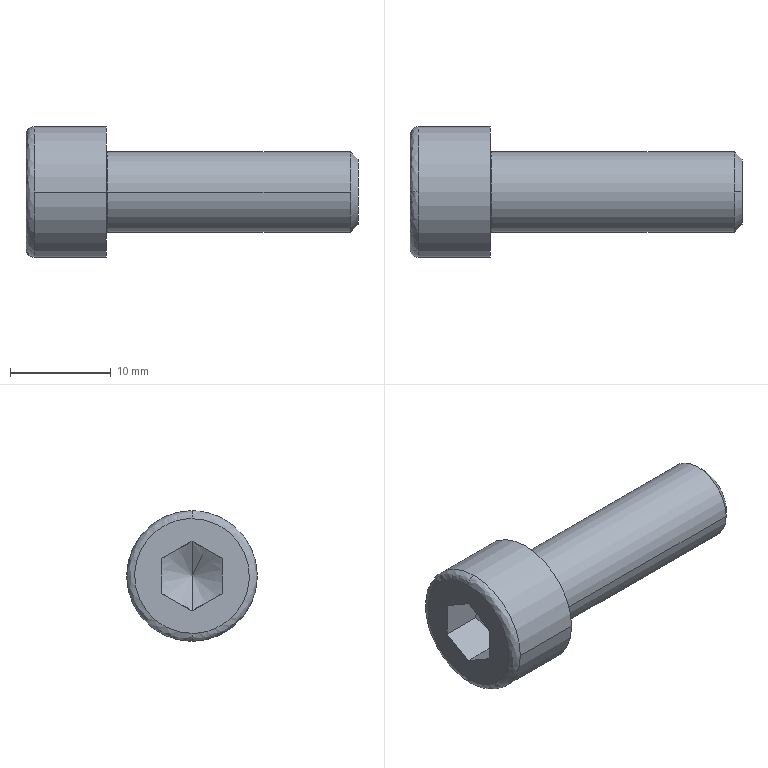Part | SolidWorks | features BaseBody 1 | 1 solid | 21 faces | box 33 x 13 x 13 mm | volume 2157 mm3 | plane 9 | spline 4 | cylinder 4 | cone 4 | commonest cylinder face diameters 8 x2 13 x2
STEP:
#1=CARTESIAN_POINT('',(0.,0.,4.1));
#2=VERTEX_POINT('',#1);
#3=CARTESIAN_POINT('',(0.,0.,-4.1));
#4=VERTEX_POINT('',#3);
#5=CARTESIAN_POINT('',(0.,0.,4.1));
#6=CARTESIAN_POINT('',(0.,0.2605,4.1));
#7=CARTESIAN_POINT('',(0.,0.6445,4.064));
#8=CARTESIAN_POINT('',(0.,1.081,3.959));
#9=CARTESIAN_POINT('',(0.,1.296,3.891));
#10=CARTESIAN_POINT('',(0.,1.388,3.858));
#11=CARTESIAN_POINT('',(0.,1.448,3.836));
#12=CARTESIAN_POINT('',(0.,1.477,3.825));
#13=CARTESIAN_POINT('',(0.,1.638,3.761));
#14=CARTESIAN_POINT('',(0.,1.826,3.675));
#15=CARTESIAN_POINT('',(0.,2.007,3.576));
#16=CARTESIAN_POINT('',(0.,2.127,3.506));
#17=CARTESIAN_POINT('',(0.,2.184,3.47));
#18=CARTESIAN_POINT('',(0.,2.48,3.277));
#19=CARTESIAN_POINT('',(0.,2.699,3.099));
#20=CARTESIAN_POINT('',(0.,2.999,2.799));
#21=CARTESIAN_POINT('',(0.,3.141,2.642));
#22=CARTESIAN_POINT('',(0.,3.27,2.475));
#23=CARTESIAN_POINT('',(0.,3.353,2.361));
#24=CARTESIAN_POINT('',(0.,3.394,2.301));
#25=CARTESIAN_POINT('',(0.,3.507,2.128));
#26=CARTESIAN_POINT('',(0.,3.612,1.949));
#27=CARTESIAN_POINT('',(0.,3.717,1.732));
#28=CARTESIAN_POINT('',(0.,3.759,1.637));
#29=CARTESIAN_POINT('',(0.,3.786,1.573));
#30=CARTESIAN_POINT('',(0.,3.8,1.539));
#31=CARTESIAN_POINT('',(0.,4.004,1.024));
#32=CARTESIAN_POINT('',(0.,4.1,0.5212));
#33=CARTESIAN_POINT('',(0.,4.1,-0.2606));
#34=CARTESIAN_POINT('',(0.,4.076,-0.5169));
#35=CARTESIAN_POINT('',(0.,4.004,-0.8942));
#36=CARTESIAN_POINT('',(0.,3.959,-1.081));
#37=CARTESIAN_POINT('',(0.,3.891,-1.296));
#38=CARTESIAN_POINT('',(0.,3.858,-1.388));
#39=CARTESIAN_POINT('',(0.,3.836,-1.449));
#40=CARTESIAN_POINT('',(0.,3.825,-1.477));
#41=CARTESIAN_POINT('',(0.,3.761,-1.638));
#42=CARTESIAN_POINT('',(0.,3.675,-1.826));
#43=CARTESIAN_POINT('',(0.,3.576,-2.007));
#44=CARTESIAN_POINT('',(0.,3.506,-2.127));
#45=CARTESIAN_POINT('',(0.,3.47,-2.184));
#46=CARTESIAN_POINT('',(0.,3.277,-2.48));
#47=CARTESIAN_POINT('',(0.,3.099,-2.699));
#48=CARTESIAN_POINT('',(0.,2.799,-2.999));
#49=CARTESIAN_POINT('',(0.,2.642,-3.141));
#50=CARTESIAN_POINT('',(0.,2.475,-3.27));
#51=CARTESIAN_POINT('',(0.,2.361,-3.353));
#52=CARTESIAN_POINT('',(0.,2.301,-3.394));
#53=CARTESIAN_POINT('',(0.,2.128,-3.507));
#54=CARTESIAN_POINT('',(0.,1.949,-3.612));
#55=CARTESIAN_POINT('',(0.,1.732,-3.717));
#56=CARTESIAN_POINT('',(0.,1.637,-3.759));
#57=CARTESIAN_POINT('',(0.,1.573,-3.786));
#58=CARTESIAN_POINT('',(0.,1.539,-3.8));
#59=CARTESIAN_POINT('',(0.,1.025,-4.004));
#60=CARTESIAN_POINT('',(0.,0.521,-4.1));
#61=CARTESIAN_POINT('',(0.,0.,-4.1));
#62=B_SPLINE_CURVE_WITH_KNOTS('',3,(#5,#6,#7,#8,#9,#10,#11,#12,#13,#14,#15,#16,#17,#18,#19,#20,#21,#22,#23,#24,#25,#26,#27,#28,#29,#30,#31,#32,#33,#34,#35,#36,#37,#38,#39,#40,#41,#42,#43,#44,#45,#46,#47,#48,#49,#50,#51,#52,#53,#54,#55,#56,#57,#58,#59,#60,#61),.UNSPECIFIED.,.F.,.F.,(4,1,1,1,2,2,1,2,2,2,1,2,2,1,1,2,2,2,2,1,1,2,2,1,2,2,2,1,2,2,1,1,2,2,4),(0.75,0.7813,0.7969,0.8047,0.8086,0.8125,0.8281,0.8359,0.8438,0.875,0.8906,0.8984,0.9063,0.9219,0.9297,0.9336,0.9375,1.,1.031,1.047,1.055,1.059,1.062,1.078,1.086,1.094,1.125,1.141,1.148,1.156,1.172,1.18,1.184,1.187,1.25),.UNSPECIFIED.);
#63=EDGE_CURVE('',#2,#4,#62,.T.);
#64=ORIENTED_EDGE('',*,*,#63,.F.);
#65=CARTESIAN_POINT('',(0.1,0.,4.));
#66=VERTEX_POINT('',#65);
#67=CARTESIAN_POINT('',(0.1,0.,4.1));
#68=DIRECTION('',(0.,-1.,0.));
#69=DIRECTION('',(0.,0.,1.));
#70=AXIS2_PLACEMENT_3D('',#67,#68,#69);
#71=CIRCLE('',#70,0.1);
#72=EDGE_CURVE('',#2,#66,#71,.T.);
#73=ORIENTED_EDGE('',*,*,#72,.T.);
#74=CARTESIAN_POINT('',(0.1,4.,0.));
#75=VERTEX_POINT('',#74);
#76=CARTESIAN_POINT('',(0.1,0.,0.));
#77=DIRECTION('',(1.,0.,0.));
#78=DIRECTION('',(0.,1.,0.));
#79=AXIS2_PLACEMENT_3D('',#76,#77,#78);
#80=CIRCLE('',#79,4.);
#81=EDGE_CURVE('',#75,#66,#80,.T.);
#82=ORIENTED_EDGE('',*,*,#81,.F.);
#83=CARTESIAN_POINT('',(0.1,0.,-4.));
#84=VERTEX_POINT('',#83);
#85=CARTESIAN_POINT('',(0.1,0.,0.));
#86=DIRECTION('',(1.,0.,0.));
#87=DIRECTION('',(0.,1.,0.));
#88=AXIS2_PLACEMENT_3D('',#85,#86,#87);
#89=CIRCLE('',#88,4.);
#90=EDGE_CURVE('',#84,#75,#89,.T.);
#91=ORIENTED_EDGE('',*,*,#90,.F.);
#92=CARTESIAN_POINT('',(0.1,0.,-4.1));
#93=DIRECTION('',(0.,1.,0.));
#94=DIRECTION('',(0.,0.,-1.));
#95=AXIS2_PLACEMENT_3D('',#92,#93,#94);
#96=CIRCLE('',#95,0.1);
#97=EDGE_CURVE('',#4,#84,#96,.T.);
#98=ORIENTED_EDGE('',*,*,#97,.F.);
#99=EDGE_LOOP('',(#64,#73,#82,#91,#98));
#100=FACE_OUTER_BOUND('',#99,.T.);
#101=CARTESIAN_POINT('',(0.,0.,-4.1));
#102=CARTESIAN_POINT('',(0.,8.2,-4.1));
#103=CARTESIAN_POINT('',(0.,8.2,4.1));
#104=CARTESIAN_POINT('',(0.,0.,4.1));
#105=CARTESIAN_POINT('',(0.,0.,-4.041));
#106=CARTESIAN_POINT('',(0.,8.083,-4.041));
#107=CARTESIAN_POINT('',(0.,8.083,4.041));
#108=CARTESIAN_POINT('',(0.,0.,4.041));
#109=CARTESIAN_POINT('',(0.04142,0.,-4.));
#110=CARTESIAN_POINT('',(0.04142,8.,-4.));
#111=CARTESIAN_POINT('',(0.04142,8.,4.));
#112=CARTESIAN_POINT('',(0.04142,0.,4.));
#113=CARTESIAN_POINT('',(0.1,0.,-4.));
#114=CARTESIAN_POINT('',(0.1,8.,-4.));
#115=CARTESIAN_POINT('',(0.1,8.,4.));
#116=CARTESIAN_POINT('',(0.1,0.,4.));
#117=(BOUNDED_SURFACE()B_SPLINE_SURFACE(3,3,((#101,#102,#103,#104),(#105,#106,#107,#108),(#109,#110,#111,#112),(#113,#114,#115,#116)),.UNSPECIFIED.,.F.,.F.,.T.)B_SPLINE_SURFACE_WITH_KNOTS((4,4),(4,4),(0.,1.),(0.,1.),.UNSPECIFIED.)GEOMETRIC_REPRESENTATION_ITEM()RATIONAL_B_SPLINE_SURFACE(((1.,0.3333,0.3333,1.),(0.8047,0.2682,0.2682,0.8047),(0.8047,0.2682,0.2682,0.8047),(1.,0.3333,0.3333,1.)))REPRESENTATION_ITEM('')SURFACE());
#118=ADVANCED_FACE('',(#100),#117,.F.);
#119=CARTESIAN_POINT('',(-7.2,0.,6.5));
#120=VERTEX_POINT('',#119);
#121=CARTESIAN_POINT('',(-7.2,-6.5,0.));
#122=VERTEX_POINT('',#121);
#123=CARTESIAN_POINT('',(-7.2,0.,0.));
#124=DIRECTION('',(1.,0.,0.));
#125=DIRECTION('',(0.,1.,0.));
#126=AXIS2_PLACEMENT_3D('',#123,#124,#125);
#127=CIRCLE('',#126,6.5);
#128=EDGE_CURVE('',#120,#122,#127,.T.);
#129=ORIENTED_EDGE('',*,*,#128,.F.);
#130=CARTESIAN_POINT('',(-8.,0.,5.7));
#131=VERTEX_POINT('',#130);
#132=CARTESIAN_POINT('',(-7.2,0.,5.7));
#133=DIRECTION('',(0.,-1.,0.));
#134=DIRECTION('',(0.,0.,1.));
#135=AXIS2_PLACEMENT_3D('',#132,#133,#134);
#136=CIRCLE('',#135,0.8);
#137=EDGE_CURVE('',#120,#131,#136,.T.);
#138=ORIENTED_EDGE('',*,*,#137,.T.);
#139=CARTESIAN_POINT('',(-8.,0.,-5.7));
#140=VERTEX_POINT('',#139);
#141=CARTESIAN_POINT('',(-8.,0.,5.7));
#142=CARTESIAN_POINT('',(-8.,-11.4,5.7));
#143=CARTESIAN_POINT('',(-8.,-11.4,-5.7));
#144=CARTESIAN_POINT('',(-8.,0.,-5.7));
#145=(BOUNDED_CURVE()B_SPLINE_CURVE(3,(#141,#142,#143,#144),.UNSPECIFIED.,.F.,.F.)B_SPLINE_CURVE_WITH_KNOTS((4,4),(0.25,0.75),.UNSPECIFIED.)CURVE()GEOMETRIC_REPRESENTATION_ITEM()RATIONAL_B_SPLINE_CURVE((1.,0.3333,0.3333,1.))REPRESENTATION_ITEM(''));
#146=EDGE_CURVE('',#131,#140,#145,.T.);
#147=ORIENTED_EDGE('',*,*,#146,.T.);
#148=CARTESIAN_POINT('',(-7.2,0.,-6.5));
#149=VERTEX_POINT('',#148);
#150=CARTESIAN_POINT('',(-7.2,0.,-5.7));
#151=DIRECTION('',(0.,1.,0.));
#152=DIRECTION('',(0.,0.,-1.));
#153=AXIS2_PLACEMENT_3D('',#150,#151,#152);
#154=CIRCLE('',#153,0.8);
#155=EDGE_CURVE('',#149,#140,#154,.T.);
#156=ORIENTED_EDGE('',*,*,#155,.F.);
#157=CARTESIAN_POINT('',(-7.2,0.,0.));
#158=DIRECTION('',(1.,0.,0.));
#159=DIRECTION('',(0.,1.,0.));
#160=AXIS2_PLACEMENT_3D('',#157,#158,#159);
#161=CIRCLE('',#160,6.5);
#162=EDGE_CURVE('',#122,#149,#161,.T.);
#163=ORIENTED_EDGE('',*,*,#162,.F.);
#164=EDGE_LOOP('',(#129,#138,#147,#156,#163));
#165=FACE_OUTER_BOUND('',#164,.T.);
#166=CARTESIAN_POINT('',(-7.2,0.,6.5));
#167=CARTESIAN_POINT('',(-7.2,-13.,6.5));
#168=CARTESIAN_POINT('',(-7.2,-13.,-6.5));
#169=CARTESIAN_POINT('',(-7.2,0.,-6.5));
#170=CARTESIAN_POINT('',(-7.669,0.,6.5));
#171=CARTESIAN_POINT('',(-7.669,-13.,6.5));
#172=CARTESIAN_POINT('',(-7.669,-13.,-6.5));
#173=CARTESIAN_POINT('',(-7.669,0.,-6.5));
#174=CARTESIAN_POINT('',(-8.,0.,6.169));
#175=CARTESIAN_POINT('',(-8.,-12.337,6.169));
#176=CARTESIAN_POINT('',(-8.,-12.337,-6.169));
#177=CARTESIAN_POINT('',(-8.,0.,-6.169));
#178=CARTESIAN_POINT('',(-8.,0.,5.7));
#179=CARTESIAN_POINT('',(-8.,-11.4,5.7));
#180=CARTESIAN_POINT('',(-8.,-11.4,-5.7));
#181=CARTESIAN_POINT('',(-8.,0.,-5.7));
#182=(BOUNDED_SURFACE()B_SPLINE_SURFACE(3,3,((#166,#167,#168,#169),(#170,#171,#172,#173),(#174,#175,#176,#177),(#178,#179,#180,#181)),.UNSPECIFIED.,.F.,.F.,.T.)B_SPLINE_SURFACE_WITH_KNOTS((4,4),(4,4),(0.,1.),(0.,1.),.UNSPECIFIED.)GEOMETRIC_REPRESENTATION_ITEM()RATIONAL_B_SPLINE_SURFACE(((1.,0.3333,0.3333,1.),(0.8047,0.2682,0.2682,0.8047),(0.8047,0.2682,0.2682,0.8047),(1.,0.3333,0.3333,1.)))REPRESENTATION_ITEM('')SURFACE());
#183=ADVANCED_FACE('',(#165),#182,.T.);
#184=ORIENTED_EDGE('',*,*,#81,.T.);
#185=CARTESIAN_POINT('',(0.1,-4.,0.));
#186=VERTEX_POINT('',#185);
#187=CARTESIAN_POINT('',(0.1,0.,0.));
#188=DIRECTION('',(1.,0.,0.));
#189=DIRECTION('',(0.,1.,0.));
#190=AXIS2_PLACEMENT_3D('',#187,#188,#189);
#191=CIRCLE('',#190,4.);
#192=EDGE_CURVE('',#66,#186,#191,.T.);
#193=ORIENTED_EDGE('',*,*,#192,.T.);
#194=CARTESIAN_POINT('',(24.233,-4.,0.));
#195=VERTEX_POINT('',#194);
#196=CARTESIAN_POINT('',(14.062,-4.,0.));
#197=DIRECTION('',(1.,0.,0.));
#198=VECTOR('',#197,1000.);
#199=LINE('',#196,#198);
#200=EDGE_CURVE('',#186,#195,#199,.T.);
#201=ORIENTED_EDGE('',*,*,#200,.T.);
#202=CARTESIAN_POINT('',(24.233,0.,4.));
#203=VERTEX_POINT('',#202);
#204=CARTESIAN_POINT('',(24.233,0.,0.));
#205=DIRECTION('',(-1.,0.,0.));
#206=DIRECTION('',(0.,1.,0.));
#207=AXIS2_PLACEMENT_3D('',#204,#205,#206);
#208=CIRCLE('',#207,4.);
#209=EDGE_CURVE('',#195,#203,#208,.T.);
#210=ORIENTED_EDGE('',*,*,#209,.T.);
#211=CARTESIAN_POINT('',(24.233,4.,0.));
#212=VERTEX_POINT('',#211);
#213=CARTESIAN_POINT('',(24.233,0.,0.));
#214=DIRECTION('',(-1.,0.,0.));
#215=DIRECTION('',(0.,1.,0.));
#216=AXIS2_PLACEMENT_3D('',#213,#214,#215);
#217=CIRCLE('',#216,4.);
#218=EDGE_CURVE('',#203,#212,#217,.T.);
#219=ORIENTED_EDGE('',*,*,#218,.T.);
#220=CARTESIAN_POINT('',(14.062,4.,0.));
#221=DIRECTION('',(1.,0.,0.));
#222=VECTOR('',#221,1000.);
#223=LINE('',#220,#222);
#224=EDGE_CURVE('',#75,#212,#223,.T.);
#225=ORIENTED_EDGE('',*,*,#224,.F.);
#226=EDGE_LOOP('',(#184,#193,#201,#210,#219,#225));
#227=FACE_OUTER_BOUND('',#226,.T.);
#228=CARTESIAN_POINT('',(14.062,0.,0.));
#229=DIRECTION('',(1.,0.,0.));
#230=DIRECTION('',(0.,1.,0.));
#231=AXIS2_PLACEMENT_3D('',#228,#229,#230);
#232=CYLINDRICAL_SURFACE('',#231,4.);
#233=ADVANCED_FACE('',(#227),#232,.T.);
#234=CARTESIAN_POINT('',(25.,0.,3.233));
#235=VERTEX_POINT('',#234);
#236=CARTESIAN_POINT('',(25.,0.,-3.233));
#237=VERTEX_POINT('',#236);
#238=CARTESIAN_POINT('',(25.,0.,0.));
#239=DIRECTION('',(-1.,0.,0.));
#240=DIRECTION('',(0.,0.,1.));
#241=AXIS2_PLACEMENT_3D('',#238,#239,#240);
#242=CIRCLE('',#241,3.233);
#243=EDGE_CURVE('',#235,#237,#242,.T.);
#244=ORIENTED_EDGE('',*,*,#243,.T.);
#245=CARTESIAN_POINT('',(24.233,0.,-4.));
#246=VERTEX_POINT('',#245);
#247=CARTESIAN_POINT('',(24.233,0.,-4.));
#248=DIRECTION('',(-0.7071,0.,-0.7071));
#249=VECTOR('',#248,1000.);
#250=LINE('',#247,#249);
#251=EDGE_CURVE('',#237,#246,#250,.T.);
#252=ORIENTED_EDGE('',*,*,#251,.T.);
#253=CARTESIAN_POINT('',(24.233,0.,0.));
#254=DIRECTION('',(-1.,0.,0.));
#255=DIRECTION('',(0.,1.,0.));
#256=AXIS2_PLACEMENT_3D('',#253,#254,#255);
#257=CIRCLE('',#256,4.);
#258=EDGE_CURVE('',#212,#246,#257,.T.);
#259=ORIENTED_EDGE('',*,*,#258,.F.);
#260=ORIENTED_EDGE('',*,*,#218,.F.);
#261=CARTESIAN_POINT('',(24.233,0.,4.));
#262=DIRECTION('',(-0.7071,0.,0.7071));
#263=VECTOR('',#262,1000.);
#264=LINE('',#261,#263);
#265=EDGE_CURVE('',#235,#203,#264,.T.);
#266=ORIENTED_EDGE('',*,*,#265,.F.);
#267=EDGE_LOOP('',(#244,#252,#259,#260,#266));
#268=FACE_OUTER_BOUND('',#267,.T.);
#269=CARTESIAN_POINT('',(24.233,0.,0.));
#270=DIRECTION('',(-1.,0.,0.));
#271=DIRECTION('',(0.,0.,1.));
#272=AXIS2_PLACEMENT_3D('',#269,#270,#271);
#273=CONICAL_SURFACE('',#272,4.,0.7854);
#274=ADVANCED_FACE('',(#268),#273,.T.);
#275=CARTESIAN_POINT('',(-7.2,6.5,0.));
#276=VERTEX_POINT('',#275);
#277=CARTESIAN_POINT('',(-7.2,0.,0.));
#278=DIRECTION('',(1.,0.,0.));
#279=DIRECTION('',(0.,1.,0.));
#280=AXIS2_PLACEMENT_3D('',#277,#278,#279);
#281=CIRCLE('',#280,6.5);
#282=EDGE_CURVE('',#276,#120,#281,.T.);
#283=ORIENTED_EDGE('',*,*,#282,.T.);
#284=ORIENTED_EDGE('',*,*,#128,.T.);
#285=CARTESIAN_POINT('',(0.,-6.5,0.));
#286=VERTEX_POINT('',#285);
#287=CARTESIAN_POINT('',(-4.,-6.5,0.));
#288=DIRECTION('',(1.,0.,0.));
#289=VECTOR('',#288,1000.);
#290=LINE('',#287,#289);
#291=EDGE_CURVE('',#122,#286,#290,.T.);
#292=ORIENTED_EDGE('',*,*,#291,.T.);
#293=CARTESIAN_POINT('',(0.,6.5,0.));
#294=VERTEX_POINT('',#293);
#295=CARTESIAN_POINT('',(0.,0.,0.));
#296=DIRECTION('',(1.,0.,0.));
#297=DIRECTION('',(0.,1.,0.));
#298=AXIS2_PLACEMENT_3D('',#295,#296,#297);
#299=CIRCLE('',#298,6.5);
#300=EDGE_CURVE('',#294,#286,#299,.T.);
#301=ORIENTED_EDGE('',*,*,#300,.F.);
#302=CARTESIAN_POINT('',(-4.,6.5,0.));
#303=DIRECTION('',(1.,0.,0.));
#304=VECTOR('',#303,1000.);
#305=LINE('',#302,#304);
#306=EDGE_CURVE('',#276,#294,#305,.T.);
#307=ORIENTED_EDGE('',*,*,#306,.F.);
#308=EDGE_LOOP('',(#283,#284,#292,#301,#307));
#309=FACE_OUTER_BOUND('',#308,.T.);
#310=CARTESIAN_POINT('',(-4.,0.,0.));
#311=DIRECTION('',(1.,0.,0.));
#312=DIRECTION('',(0.,1.,0.));
#313=AXIS2_PLACEMENT_3D('',#310,#311,#312);
#314=CYLINDRICAL_SURFACE('',#313,6.5);
#315=ADVANCED_FACE('',(#309),#314,.T.);
#316=CARTESIAN_POINT('',(-2.,0.,0.));
#317=VERTEX_POINT('',#316);
#318=CARTESIAN_POINT('',(-4.,0.,3.464));
#319=VERTEX_POINT('',#318);
#320=CARTESIAN_POINT('',(-4.012,0.,3.485));
#321=DIRECTION('',(-0.5,0.,0.866));
#322=VECTOR('',#321,1000.);
#323=LINE('',#320,#322);
#324=EDGE_CURVE('',#317,#319,#323,.T.);
#325=ORIENTED_EDGE('',*,*,#324,.F.);
#326=CARTESIAN_POINT('',(-4.,0.,-3.464));
#327=VERTEX_POINT('',#326);
#328=CARTESIAN_POINT('',(-4.012,0.,-3.485));
#329=DIRECTION('',(-0.5,0.,-0.866));
#330=VECTOR('',#329,1000.);
#331=LINE('',#328,#330);
#332=EDGE_CURVE('',#317,#327,#331,.T.);
#333=ORIENTED_EDGE('',*,*,#332,.T.);
#334=CARTESIAN_POINT('',(-4.,-3.,-1.732));
#335=VERTEX_POINT('',#334);
#336=CARTESIAN_POINT('',(-4.,0.,-3.464));
#337=CARTESIAN_POINT('',(-3.837,-0.4898,-3.181));
#338=CARTESIAN_POINT('',(-3.732,-0.987,-2.894));
#339=CARTESIAN_POINT('',(-3.732,-1.752,-2.452));
#340=CARTESIAN_POINT('',(-3.757,-2.007,-2.305));
#341=CARTESIAN_POINT('',(-3.851,-2.507,-2.016));
#342=CARTESIAN_POINT('',(-3.918,-2.755,-1.874));
#343=CARTESIAN_POINT('',(-4.,-3.,-1.732));
#344=B_SPLINE_CURVE_WITH_KNOTS('',3,(#336,#337,#338,#339,#340,#341,#342,#343),.UNSPECIFIED.,.F.,.F.,(4,2,2,4),(0.,0.001749,0.002624,0.003499),.UNSPECIFIED.);
#345=EDGE_CURVE('',#327,#335,#344,.T.);
#346=ORIENTED_EDGE('',*,*,#345,.T.);
#347=CARTESIAN_POINT('',(-4.,-3.,1.732));
#348=VERTEX_POINT('',#347);
#349=CARTESIAN_POINT('',(-4.,-3.,-1.732));
#350=CARTESIAN_POINT('',(-3.837,-3.,-1.166));
#351=CARTESIAN_POINT('',(-3.732,-3.,-0.5923));
#352=CARTESIAN_POINT('',(-3.732,-3.,0.2912));
#353=CARTESIAN_POINT('',(-3.757,-3.,0.5854));
#354=CARTESIAN_POINT('',(-3.851,-3.,1.163));
#355=CARTESIAN_POINT('',(-3.918,-3.,1.449));
#356=CARTESIAN_POINT('',(-4.,-3.,1.732));
#357=B_SPLINE_CURVE_WITH_KNOTS('',3,(#349,#350,#351,#352,#353,#354,#355,#356),.UNSPECIFIED.,.F.,.F.,(4,2,2,4),(0.,0.001749,0.002624,0.003499),.UNSPECIFIED.);
#358=EDGE_CURVE('',#335,#348,#357,.T.);
#359=ORIENTED_EDGE('',*,*,#358,.T.);
#360=CARTESIAN_POINT('',(-4.,-3.,1.732));
#361=CARTESIAN_POINT('',(-3.837,-2.51,2.015));
#362=CARTESIAN_POINT('',(-3.732,-2.013,2.302));
#363=CARTESIAN_POINT('',(-3.732,-1.248,2.744));
#364=CARTESIAN_POINT('',(-3.757,-0.993,2.891));
#365=CARTESIAN_POINT('',(-3.851,-0.4925,3.18));
#366=CARTESIAN_POINT('',(-3.918,-0.2452,3.323));
#367=CARTESIAN_POINT('',(-4.,0.,3.464));
#368=B_SPLINE_CURVE_WITH_KNOTS('',3,(#360,#361,#362,#363,#364,#365,#366,#367),.UNSPECIFIED.,.F.,.F.,(4,2,2,4),(0.,0.001749,0.002624,0.003499),.UNSPECIFIED.);
#369=EDGE_CURVE('',#348,#319,#368,.T.);
#370=ORIENTED_EDGE('',*,*,#369,.T.);
#371=EDGE_LOOP('',(#325,#333,#346,#359,#370));
#372=FACE_OUTER_BOUND('',#371,.T.);
#373=CARTESIAN_POINT('',(-4.012,0.,0.));
#374=DIRECTION('',(-1.,0.,0.));
#375=DIRECTION('',(0.,0.,1.));
#376=AXIS2_PLACEMENT_3D('',#373,#374,#375);
#377=CONICAL_SURFACE('',#376,3.485,1.047);
#378=ADVANCED_FACE('',(#372),#377,.F.);
#379=ORIENTED_EDGE('',*,*,#200,.F.);
#380=CARTESIAN_POINT('',(0.1,0.,0.));
#381=DIRECTION('',(1.,0.,0.));
#382=DIRECTION('',(0.,1.,0.));
#383=AXIS2_PLACEMENT_3D('',#380,#381,#382);
#384=CIRCLE('',#383,4.);
#385=EDGE_CURVE('',#186,#84,#384,.T.);
#386=ORIENTED_EDGE('',*,*,#385,.T.);
#387=ORIENTED_EDGE('',*,*,#90,.T.);
#388=ORIENTED_EDGE('',*,*,#224,.T.);
#389=ORIENTED_EDGE('',*,*,#258,.T.);
#390=CARTESIAN_POINT('',(24.233,0.,0.));
#391=DIRECTION('',(-1.,0.,0.));
#392=DIRECTION('',(0.,1.,0.));
#393=AXIS2_PLACEMENT_3D('',#390,#391,#392);
#394=CIRCLE('',#393,4.);
#395=EDGE_CURVE('',#246,#195,#394,.T.);
#396=ORIENTED_EDGE('',*,*,#395,.T.);
#397=EDGE_LOOP('',(#379,#386,#387,#388,#389,#396));
#398=FACE_OUTER_BOUND('',#397,.T.);
#399=CARTESIAN_POINT('',(14.062,0.,0.));
#400=DIRECTION('',(1.,0.,0.));
#401=DIRECTION('',(0.,1.,0.));
#402=AXIS2_PLACEMENT_3D('',#399,#400,#401);
#403=CYLINDRICAL_SURFACE('',#402,4.);
#404=ADVANCED_FACE('',(#398),#403,.T.);
#405=ORIENTED_EDGE('',*,*,#72,.F.);
#406=CARTESIAN_POINT('',(0.,0.,-4.1));
#407=CARTESIAN_POINT('',(0.,-0.2605,-4.1));
#408=CARTESIAN_POINT('',(0.,-0.6445,-4.064));
#409=CARTESIAN_POINT('',(0.,-1.081,-3.959));
#410=CARTESIAN_POINT('',(0.,-1.296,-3.891));
#411=CARTESIAN_POINT('',(0.,-1.388,-3.858));
#412=CARTESIAN_POINT('',(0.,-1.448,-3.836));
#413=CARTESIAN_POINT('',(0.,-1.477,-3.825));
#414=CARTESIAN_POINT('',(0.,-1.638,-3.761));
#415=CARTESIAN_POINT('',(0.,-1.826,-3.675));
#416=CARTESIAN_POINT('',(0.,-2.007,-3.576));
#417=CARTESIAN_POINT('',(0.,-2.127,-3.506));
#418=CARTESIAN_POINT('',(0.,-2.184,-3.47));
#419=CARTESIAN_POINT('',(0.,-2.48,-3.277));
#420=CARTESIAN_POINT('',(0.,-2.699,-3.099));
#421=CARTESIAN_POINT('',(0.,-2.999,-2.799));
#422=CARTESIAN_POINT('',(0.,-3.141,-2.642));
#423=CARTESIAN_POINT('',(0.,-3.27,-2.475));
#424=CARTESIAN_POINT('',(0.,-3.353,-2.361));
#425=CARTESIAN_POINT('',(0.,-3.394,-2.301));
#426=CARTESIAN_POINT('',(0.,-3.507,-2.128));
#427=CARTESIAN_POINT('',(0.,-3.612,-1.949));
#428=CARTESIAN_POINT('',(0.,-3.717,-1.732));
#429=CARTESIAN_POINT('',(0.,-3.759,-1.637));
#430=CARTESIAN_POINT('',(0.,-3.786,-1.573));
#431=CARTESIAN_POINT('',(0.,-3.8,-1.539));
#432=CARTESIAN_POINT('',(0.,-4.004,-1.025));
#433=CARTESIAN_POINT('',(0.,-4.1,-0.521));
#434=CARTESIAN_POINT('',(0.,-4.1,0.2605));
#435=CARTESIAN_POINT('',(0.,-4.064,0.6445));
#436=CARTESIAN_POINT('',(0.,-3.959,1.081));
#437=CARTESIAN_POINT('',(0.,-3.891,1.296));
#438=CARTESIAN_POINT('',(0.,-3.858,1.388));
#439=CARTESIAN_POINT('',(0.,-3.836,1.448));
#440=CARTESIAN_POINT('',(0.,-3.825,1.477));
#441=CARTESIAN_POINT('',(0.,-3.761,1.638));
#442=CARTESIAN_POINT('',(0.,-3.675,1.826));
#443=CARTESIAN_POINT('',(0.,-3.576,2.007));
#444=CARTESIAN_POINT('',(0.,-3.506,2.127));
#445=CARTESIAN_POINT('',(0.,-3.47,2.184));
#446=CARTESIAN_POINT('',(0.,-3.277,2.48));
#447=CARTESIAN_POINT('',(0.,-3.099,2.699));
#448=CARTESIAN_POINT('',(0.,-2.799,2.999));
#449=CARTESIAN_POINT('',(0.,-2.642,3.141));
#450=CARTESIAN_POINT('',(0.,-2.475,3.27));
#451=CARTESIAN_POINT('',(0.,-2.361,3.353));
#452=CARTESIAN_POINT('',(0.,-2.301,3.394));
#453=CARTESIAN_POINT('',(0.,-2.128,3.507));
#454=CARTESIAN_POINT('',(0.,-1.949,3.612));
#455=CARTESIAN_POINT('',(0.,-1.732,3.717));
#456=CARTESIAN_POINT('',(0.,-1.637,3.759));
#457=CARTESIAN_POINT('',(0.,-1.573,3.786));
#458=CARTESIAN_POINT('',(0.,-1.539,3.8));
#459=CARTESIAN_POINT('',(0.,-1.025,4.004));
#460=CARTESIAN_POINT('',(0.,-0.521,4.1));
#461=CARTESIAN_POINT('',(0.,0.,4.1));
#462=B_SPLINE_CURVE_WITH_KNOTS('',3,(#406,#407,#408,#409,#410,#411,#412,#413,#414,#415,#416,#417,#418,#419,#420,#421,#422,#423,#424,#425,#426,#427,#428,#429,#430,#431,#432,#433,#434,#435,#436,#437,#438,#439,#440,#441,#442,#443,#444,#445,#446,#447,#448,#449,#450,#451,#452,#453,#454,#455,#456,#457,#458,#459,#460,#461),.UNSPECIFIED.,.F.,.F.,(4,1,1,1,2,2,1,2,2,2,1,2,2,1,1,2,2,2,1,1,1,2,2,1,2,2,2,1,2,2,1,1,2,2,4),(0.25,0.2812,0.2969,0.3047,0.3086,0.3125,0.3281,0.3359,0.3437,0.375,0.3906,0.3984,0.4062,0.4219,0.4297,0.4336,0.4375,0.5,0.5312,0.5469,0.5547,0.5586,0.5625,0.5781,0.5859,0.5937,0.625,0.6406,0.6484,0.6562,0.6719,0.6797,0.6836,0.6875,0.75),.UNSPECIFIED.);
#463=EDGE_CURVE('',#4,#2,#462,.T.);
#464=ORIENTED_EDGE('',*,*,#463,.F.);
#465=ORIENTED_EDGE('',*,*,#97,.T.);
#466=ORIENTED_EDGE('',*,*,#385,.F.);
#467=ORIENTED_EDGE('',*,*,#192,.F.);
#468=EDGE_LOOP('',(#405,#464,#465,#466,#467));
#469=FACE_OUTER_BOUND('',#468,.T.);
#470=CARTESIAN_POINT('',(0.,0.,4.1));
#471=CARTESIAN_POINT('',(0.,-8.2,4.1));
#472=CARTESIAN_POINT('',(0.,-8.2,-4.1));
#473=CARTESIAN_POINT('',(0.,0.,-4.1));
#474=CARTESIAN_POINT('',(0.,0.,4.041));
#475=CARTESIAN_POINT('',(0.,-8.083,4.041));
#476=CARTESIAN_POINT('',(0.,-8.083,-4.041));
#477=CARTESIAN_POINT('',(0.,0.,-4.041));
#478=CARTESIAN_POINT('',(0.04142,0.,4.));
#479=CARTESIAN_POINT('',(0.04142,-8.,4.));
#480=CARTESIAN_POINT('',(0.04142,-8.,-4.));
#481=CARTESIAN_POINT('',(0.04142,0.,-4.));
#482=CARTESIAN_POINT('',(0.1,0.,4.));
#483=CARTESIAN_POINT('',(0.1,-8.,4.));
#484=CARTESIAN_POINT('',(0.1,-8.,-4.));
#485=CARTESIAN_POINT('',(0.1,0.,-4.));
#486=(BOUNDED_SURFACE()B_SPLINE_SURFACE(3,3,((#470,#471,#472,#473),(#474,#475,#476,#477),(#478,#479,#480,#481),(#482,#483,#484,#485)),.UNSPECIFIED.,.F.,.F.,.F.)B_SPLINE_SURFACE_WITH_KNOTS((4,4),(4,4),(0.,1.),(0.,1.),.UNSPECIFIED.)GEOMETRIC_REPRESENTATION_ITEM()RATIONAL_B_SPLINE_SURFACE(((1.,0.3333,0.3333,1.),(0.8047,0.2682,0.2682,0.8047),(0.8047,0.2682,0.2682,0.8047),(1.,0.3333,0.3333,1.)))REPRESENTATION_ITEM('')SURFACE());
#487=ADVANCED_FACE('',(#469),#486,.F.);
#488=ORIENTED_EDGE('',*,*,#251,.F.);
#489=CARTESIAN_POINT('',(25.,0.,0.));
#490=DIRECTION('',(-1.,0.,0.));
#491=DIRECTION('',(0.,0.,1.));
#492=AXIS2_PLACEMENT_3D('',#489,#490,#491);
#493=CIRCLE('',#492,3.233);
#494=EDGE_CURVE('',#237,#235,#493,.T.);
#495=ORIENTED_EDGE('',*,*,#494,.T.);
#496=ORIENTED_EDGE('',*,*,#265,.T.);
#497=ORIENTED_EDGE('',*,*,#209,.F.);
#498=ORIENTED_EDGE('',*,*,#395,.F.);
#499=EDGE_LOOP('',(#488,#495,#496,#497,#498));
#500=FACE_OUTER_BOUND('',#499,.T.);
#501=CARTESIAN_POINT('',(24.233,0.,0.));
#502=DIRECTION('',(-1.,0.,0.));
#503=DIRECTION('',(0.,0.,1.));
#504=AXIS2_PLACEMENT_3D('',#501,#502,#503);
#505=CONICAL_SURFACE('',#504,4.,0.7854);
#506=ADVANCED_FACE('',(#500),#505,.T.);
#507=ORIENTED_EDGE('',*,*,#463,.T.);
#508=ORIENTED_EDGE('',*,*,#63,.T.);
#509=EDGE_LOOP('',(#507,#508));
#510=FACE_BOUND('',#509,.T.);
#511=ORIENTED_EDGE('',*,*,#300,.T.);
#512=CARTESIAN_POINT('',(0.,0.,0.));
#513=DIRECTION('',(1.,0.,0.));
#514=DIRECTION('',(0.,1.,0.));
#515=AXIS2_PLACEMENT_3D('',#512,#513,#514);
#516=CIRCLE('',#515,6.5);
#517=EDGE_CURVE('',#286,#294,#516,.T.);
#518=ORIENTED_EDGE('',*,*,#517,.T.);
#519=EDGE_LOOP('',(#511,#518));
#520=FACE_OUTER_BOUND('',#519,.T.);
#521=CARTESIAN_POINT('',(0.,5.25,0.));
#522=DIRECTION('',(1.,0.,0.));
#523=DIRECTION('',(0.,1.,0.));
#524=AXIS2_PLACEMENT_3D('',#521,#522,#523);
#525=PLANE('',#524);
#526=ADVANCED_FACE('',(#510,#520),#525,.T.);
#527=ORIENTED_EDGE('',*,*,#243,.F.);
#528=ORIENTED_EDGE('',*,*,#494,.F.);
#529=EDGE_LOOP('',(#527,#528));
#530=FACE_OUTER_BOUND('',#529,.T.);
#531=CARTESIAN_POINT('',(25.,2.,0.));
#532=DIRECTION('',(1.,0.,0.));
#533=DIRECTION('',(0.,1.,0.));
#534=AXIS2_PLACEMENT_3D('',#531,#532,#533);
#535=PLANE('',#534);
#536=ADVANCED_FACE('',(#530),#535,.T.);
#537=ORIENTED_EDGE('',*,*,#291,.F.);
#538=ORIENTED_EDGE('',*,*,#162,.T.);
#539=CARTESIAN_POINT('',(-7.2,0.,0.));
#540=DIRECTION('',(1.,0.,0.));
#541=DIRECTION('',(0.,1.,0.));
#542=AXIS2_PLACEMENT_3D('',#539,#540,#541);
#543=CIRCLE('',#542,6.5);
#544=EDGE_CURVE('',#149,#276,#543,.T.);
#545=ORIENTED_EDGE('',*,*,#544,.T.);
#546=ORIENTED_EDGE('',*,*,#306,.T.);
#547=ORIENTED_EDGE('',*,*,#517,.F.);
#548=EDGE_LOOP('',(#537,#538,#545,#546,#547));
#549=FACE_OUTER_BOUND('',#548,.T.);
#550=CARTESIAN_POINT('',(-4.,0.,0.));
#551=DIRECTION('',(1.,0.,0.));
#552=DIRECTION('',(0.,1.,0.));
#553=AXIS2_PLACEMENT_3D('',#550,#551,#552);
#554=CYLINDRICAL_SURFACE('',#553,6.5);
#555=ADVANCED_FACE('',(#549),#554,.T.);
#556=ORIENTED_EDGE('',*,*,#137,.F.);
#557=ORIENTED_EDGE('',*,*,#282,.F.);
#558=ORIENTED_EDGE('',*,*,#544,.F.);
#559=ORIENTED_EDGE('',*,*,#155,.T.);
#560=CARTESIAN_POINT('',(-8.,0.,-5.7));
#561=CARTESIAN_POINT('',(-8.,11.4,-5.7));
#562=CARTESIAN_POINT('',(-8.,11.4,5.7));
#563=CARTESIAN_POINT('',(-8.,0.,5.7));
#564=(BOUNDED_CURVE()B_SPLINE_CURVE(3,(#560,#561,#562,#563),.UNSPECIFIED.,.F.,.T.)B_SPLINE_CURVE_WITH_KNOTS((4,4),(0.75,1.25),.UNSPECIFIED.)CURVE()GEOMETRIC_REPRESENTATION_ITEM()RATIONAL_B_SPLINE_CURVE((1.,0.3333,0.3333,1.))REPRESENTATION_ITEM(''));
#565=EDGE_CURVE('',#140,#131,#564,.T.);
#566=ORIENTED_EDGE('',*,*,#565,.T.);
#567=EDGE_LOOP('',(#556,#557,#558,#559,#566));
#568=FACE_OUTER_BOUND('',#567,.T.);
#569=CARTESIAN_POINT('',(-7.2,0.,-6.5));
#570=CARTESIAN_POINT('',(-7.2,13.,-6.5));
#571=CARTESIAN_POINT('',(-7.2,13.,6.5));
#572=CARTESIAN_POINT('',(-7.2,0.,6.5));
#573=CARTESIAN_POINT('',(-7.669,0.,-6.5));
#574=CARTESIAN_POINT('',(-7.669,13.,-6.5));
#575=CARTESIAN_POINT('',(-7.669,13.,6.5));
#576=CARTESIAN_POINT('',(-7.669,0.,6.5));
#577=CARTESIAN_POINT('',(-8.,0.,-6.169));
#578=CARTESIAN_POINT('',(-8.,12.337,-6.169));
#579=CARTESIAN_POINT('',(-8.,12.337,6.169));
#580=CARTESIAN_POINT('',(-8.,0.,6.169));
#581=CARTESIAN_POINT('',(-8.,0.,-5.7));
#582=CARTESIAN_POINT('',(-8.,11.4,-5.7));
#583=CARTESIAN_POINT('',(-8.,11.4,5.7));
#584=CARTESIAN_POINT('',(-8.,0.,5.7));
#585=(BOUNDED_SURFACE()B_SPLINE_SURFACE(3,3,((#569,#570,#571,#572),(#573,#574,#575,#576),(#577,#578,#579,#580),(#581,#582,#583,#584)),.UNSPECIFIED.,.F.,.F.,.T.)B_SPLINE_SURFACE_WITH_KNOTS((4,4),(4,4),(0.,1.),(0.,1.),.UNSPECIFIED.)GEOMETRIC_REPRESENTATION_ITEM()RATIONAL_B_SPLINE_SURFACE(((1.,0.3333,0.3333,1.),(0.8047,0.2682,0.2682,0.8047),(0.8047,0.2682,0.2682,0.8047),(1.,0.3333,0.3333,1.)))REPRESENTATION_ITEM('')SURFACE());
#586=ADVANCED_FACE('',(#568),#585,.T.);
#587=CARTESIAN_POINT('',(-8.,-3.,-1.732));
#588=VERTEX_POINT('',#587);
#589=CARTESIAN_POINT('',(-8.,0.,-3.464));
#590=VERTEX_POINT('',#589);
#591=CARTESIAN_POINT('',(-8.,-3.,-1.732));
#592=DIRECTION('',(0.,0.866,-0.5));
#593=VECTOR('',#592,1000.);
#594=LINE('',#591,#593);
#595=EDGE_CURVE('',#588,#590,#594,.T.);
#596=ORIENTED_EDGE('',*,*,#595,.T.);
#597=CARTESIAN_POINT('',(-8.,3.,-1.732));
#598=VERTEX_POINT('',#597);
#599=CARTESIAN_POINT('',(-8.,0.,-3.464));
#600=DIRECTION('',(0.,0.866,0.5));
#601=VECTOR('',#600,1000.);
#602=LINE('',#599,#601);
#603=EDGE_CURVE('',#590,#598,#602,.T.);
#604=ORIENTED_EDGE('',*,*,#603,.T.);
#605=CARTESIAN_POINT('',(-8.,3.,1.732));
#606=VERTEX_POINT('',#605);
#607=CARTESIAN_POINT('',(-8.,3.,0.));
#608=DIRECTION('',(0.,0.,1.));
#609=VECTOR('',#608,1000.);
#610=LINE('',#607,#609);
#611=EDGE_CURVE('',#598,#606,#610,.T.);
#612=ORIENTED_EDGE('',*,*,#611,.T.);
#613=CARTESIAN_POINT('',(-8.,0.,3.464));
#614=VERTEX_POINT('',#613);
#615=CARTESIAN_POINT('',(-8.,3.,1.732));
#616=DIRECTION('',(0.,-0.866,0.5));
#617=VECTOR('',#616,1000.);
#618=LINE('',#615,#617);
#619=EDGE_CURVE('',#606,#614,#618,.T.);
#620=ORIENTED_EDGE('',*,*,#619,.T.);
#621=CARTESIAN_POINT('',(-8.,-3.,1.732));
#622=VERTEX_POINT('',#621);
#623=CARTESIAN_POINT('',(-8.,0.,3.464));
#624=DIRECTION('',(0.,-0.866,-0.5));
#625=VECTOR('',#624,1000.);
#626=LINE('',#623,#625);
#627=EDGE_CURVE('',#614,#622,#626,.T.);
#628=ORIENTED_EDGE('',*,*,#627,.T.);
#629=CARTESIAN_POINT('',(-8.,-3.,0.));
#630=DIRECTION('',(0.,0.,-1.));
#631=VECTOR('',#630,1000.);
#632=LINE('',#629,#631);
#633=EDGE_CURVE('',#622,#588,#632,.T.);
#634=ORIENTED_EDGE('',*,*,#633,.T.);
#635=EDGE_LOOP('',(#596,#604,#612,#620,#628,#634));
#636=FACE_BOUND('',#635,.T.);
#637=ORIENTED_EDGE('',*,*,#565,.F.);
#638=ORIENTED_EDGE('',*,*,#146,.F.);
#639=EDGE_LOOP('',(#637,#638));
#640=FACE_OUTER_BOUND('',#639,.T.);
#641=CARTESIAN_POINT('',(-8.,4.982,0.));
#642=DIRECTION('',(-1.,0.,0.));
#643=DIRECTION('',(0.,-1.,0.));
#644=AXIS2_PLACEMENT_3D('',#641,#642,#643);
#645=PLANE('',#644);
#646=ADVANCED_FACE('',(#636,#640),#645,.T.);
#647=CARTESIAN_POINT('',(-4.,3.,-1.732));
#648=VERTEX_POINT('',#647);
#649=CARTESIAN_POINT('',(-8.,3.,-1.732));
#650=DIRECTION('',(1.,0.,0.));
#651=VECTOR('',#650,1000.);
#652=LINE('',#649,#651);
#653=EDGE_CURVE('',#598,#648,#652,.T.);
#654=ORIENTED_EDGE('',*,*,#653,.F.);
#655=ORIENTED_EDGE('',*,*,#603,.F.);
#656=CARTESIAN_POINT('',(-8.,0.,-3.464));
#657=DIRECTION('',(-1.,0.,0.));
#658=VECTOR('',#657,1000.);
#659=LINE('',#656,#658);
#660=EDGE_CURVE('',#327,#590,#659,.T.);
#661=ORIENTED_EDGE('',*,*,#660,.F.);
#662=CARTESIAN_POINT('',(-4.,3.,-1.732));
#663=CARTESIAN_POINT('',(-3.837,2.51,-2.015));
#664=CARTESIAN_POINT('',(-3.732,2.013,-2.302));
#665=CARTESIAN_POINT('',(-3.732,1.248,-2.744));
#666=CARTESIAN_POINT('',(-3.757,0.993,-2.891));
#667=CARTESIAN_POINT('',(-3.851,0.4925,-3.18));
#668=CARTESIAN_POINT('',(-3.918,0.2452,-3.323));
#669=CARTESIAN_POINT('',(-4.,0.,-3.464));
#670=B_SPLINE_CURVE_WITH_KNOTS('',3,(#662,#663,#664,#665,#666,#667,#668,#669),.UNSPECIFIED.,.F.,.F.,(4,2,2,4),(0.,0.001749,0.002624,0.003499),.UNSPECIFIED.);
#671=EDGE_CURVE('',#648,#327,#670,.T.);
#672=ORIENTED_EDGE('',*,*,#671,.F.);
#673=EDGE_LOOP('',(#654,#655,#661,#672));
#674=FACE_OUTER_BOUND('',#673,.T.);
#675=CARTESIAN_POINT('',(-8.,3.,-1.732));
#676=DIRECTION('',(0.,0.5,-0.866));
#677=DIRECTION('',(0.,0.866,0.5));
#678=AXIS2_PLACEMENT_3D('',#675,#676,#677);
#679=PLANE('',#678);
#680=ADVANCED_FACE('',(#674),#679,.F.);
#681=ORIENTED_EDGE('',*,*,#660,.T.);
#682=ORIENTED_EDGE('',*,*,#595,.F.);
#683=CARTESIAN_POINT('',(-8.,-3.,-1.732));
#684=DIRECTION('',(-1.,0.,0.));
#685=VECTOR('',#684,1000.);
#686=LINE('',#683,#685);
#687=EDGE_CURVE('',#335,#588,#686,.T.);
#688=ORIENTED_EDGE('',*,*,#687,.F.);
#689=ORIENTED_EDGE('',*,*,#345,.F.);
#690=EDGE_LOOP('',(#681,#682,#688,#689));
#691=FACE_OUTER_BOUND('',#690,.T.);
#692=CARTESIAN_POINT('',(-8.,0.,-3.464));
#693=DIRECTION('',(0.,-0.5,-0.866));
#694=DIRECTION('',(0.,0.866,-0.5));
#695=AXIS2_PLACEMENT_3D('',#692,#693,#694);
#696=PLANE('',#695);
#697=ADVANCED_FACE('',(#691),#696,.F.);
#698=ORIENTED_EDGE('',*,*,#687,.T.);
#699=ORIENTED_EDGE('',*,*,#633,.F.);
#700=CARTESIAN_POINT('',(-8.,-3.,1.732));
#701=DIRECTION('',(-1.,0.,0.));
#702=VECTOR('',#701,1000.);
#703=LINE('',#700,#702);
#704=EDGE_CURVE('',#348,#622,#703,.T.);
#705=ORIENTED_EDGE('',*,*,#704,.F.);
#706=ORIENTED_EDGE('',*,*,#358,.F.);
#707=EDGE_LOOP('',(#698,#699,#705,#706));
#708=FACE_OUTER_BOUND('',#707,.T.);
#709=CARTESIAN_POINT('',(-8.,-3.,-1.732));
#710=DIRECTION('',(0.,-1.,0.));
#711=DIRECTION('',(0.,0.,-1.));
#712=AXIS2_PLACEMENT_3D('',#709,#710,#711);
#713=PLANE('',#712);
#714=ADVANCED_FACE('',(#708),#713,.F.);
#715=ORIENTED_EDGE('',*,*,#704,.T.);
#716=ORIENTED_EDGE('',*,*,#627,.F.);
#717=CARTESIAN_POINT('',(-8.,0.,3.464));
#718=DIRECTION('',(-1.,0.,0.));
#719=VECTOR('',#718,1000.);
#720=LINE('',#717,#719);
#721=EDGE_CURVE('',#319,#614,#720,.T.);
#722=ORIENTED_EDGE('',*,*,#721,.F.);
#723=ORIENTED_EDGE('',*,*,#369,.F.);
#724=EDGE_LOOP('',(#715,#716,#722,#723));
#725=FACE_OUTER_BOUND('',#724,.T.);
#726=CARTESIAN_POINT('',(-8.,-3.,1.732));
#727=DIRECTION('',(0.,-0.5,0.866));
#728=DIRECTION('',(0.,-0.866,-0.5));
#729=AXIS2_PLACEMENT_3D('',#726,#727,#728);
#730=PLANE('',#729);
#731=ADVANCED_FACE('',(#725),#730,.F.);
#732=ORIENTED_EDGE('',*,*,#721,.T.);
#733=ORIENTED_EDGE('',*,*,#619,.F.);
#734=CARTESIAN_POINT('',(-4.,3.,1.732));
#735=VERTEX_POINT('',#734);
#736=CARTESIAN_POINT('',(-8.,3.,1.732));
#737=DIRECTION('',(-1.,0.,0.));
#738=VECTOR('',#737,1000.);
#739=LINE('',#736,#738);
#740=EDGE_CURVE('',#735,#606,#739,.T.);
#741=ORIENTED_EDGE('',*,*,#740,.F.);
#742=CARTESIAN_POINT('',(-4.,0.,3.464));
#743=CARTESIAN_POINT('',(-3.837,0.4898,3.181));
#744=CARTESIAN_POINT('',(-3.732,0.987,2.894));
#745=CARTESIAN_POINT('',(-3.732,1.752,2.452));
#746=CARTESIAN_POINT('',(-3.757,2.007,2.305));
#747=CARTESIAN_POINT('',(-3.851,2.507,2.016));
#748=CARTESIAN_POINT('',(-3.918,2.755,1.874));
#749=CARTESIAN_POINT('',(-4.,3.,1.732));
#750=B_SPLINE_CURVE_WITH_KNOTS('',3,(#742,#743,#744,#745,#746,#747,#748,#749),.UNSPECIFIED.,.F.,.F.,(4,2,2,4),(0.,0.001749,0.002624,0.003499),.UNSPECIFIED.);
#751=EDGE_CURVE('',#319,#735,#750,.T.);
#752=ORIENTED_EDGE('',*,*,#751,.F.);
#753=EDGE_LOOP('',(#732,#733,#741,#752));
#754=FACE_OUTER_BOUND('',#753,.T.);
#755=CARTESIAN_POINT('',(-8.,0.,3.464));
#756=DIRECTION('',(0.,0.5,0.866));
#757=DIRECTION('',(0.,-0.866,0.5));
#758=AXIS2_PLACEMENT_3D('',#755,#756,#757);
#759=PLANE('',#758);
#760=ADVANCED_FACE('',(#754),#759,.F.);
#761=ORIENTED_EDGE('',*,*,#740,.T.);
#762=ORIENTED_EDGE('',*,*,#611,.F.);
#763=ORIENTED_EDGE('',*,*,#653,.T.);
#764=CARTESIAN_POINT('',(-4.,3.,1.732));
#765=CARTESIAN_POINT('',(-3.837,3.,1.166));
#766=CARTESIAN_POINT('',(-3.732,3.,0.5923));
#767=CARTESIAN_POINT('',(-3.732,3.,-0.2912));
#768=CARTESIAN_POINT('',(-3.757,3.,-0.5854));
#769=CARTESIAN_POINT('',(-3.851,3.,-1.163));
#770=CARTESIAN_POINT('',(-3.918,3.,-1.449));
#771=CARTESIAN_POINT('',(-4.,3.,-1.732));
#772=B_SPLINE_CURVE_WITH_KNOTS('',3,(#764,#765,#766,#767,#768,#769,#770,#771),.UNSPECIFIED.,.F.,.F.,(4,2,2,4),(0.,0.001749,0.002624,0.003499),.UNSPECIFIED.);
#773=EDGE_CURVE('',#735,#648,#772,.T.);
#774=ORIENTED_EDGE('',*,*,#773,.F.);
#775=EDGE_LOOP('',(#761,#762,#763,#774));
#776=FACE_OUTER_BOUND('',#775,.T.);
#777=CARTESIAN_POINT('',(-8.,3.,1.732));
#778=DIRECTION('',(0.,1.,0.));
#779=DIRECTION('',(0.,0.,1.));
#780=AXIS2_PLACEMENT_3D('',#777,#778,#779);
#781=PLANE('',#780);
#782=ADVANCED_FACE('',(#776),#781,.F.);
#783=ORIENTED_EDGE('',*,*,#332,.F.);
#784=ORIENTED_EDGE('',*,*,#324,.T.);
#785=ORIENTED_EDGE('',*,*,#751,.T.);
#786=ORIENTED_EDGE('',*,*,#773,.T.);
#787=ORIENTED_EDGE('',*,*,#671,.T.);
#788=EDGE_LOOP('',(#783,#784,#785,#786,#787));
#789=FACE_OUTER_BOUND('',#788,.T.);
#790=CARTESIAN_POINT('',(-4.012,0.,0.));
#791=DIRECTION('',(-1.,0.,0.));
#792=DIRECTION('',(0.,0.,1.));
#793=AXIS2_PLACEMENT_3D('',#790,#791,#792);
#794=CONICAL_SURFACE('',#793,3.485,1.047);
#795=ADVANCED_FACE('',(#789),#794,.F.);
#796=CLOSED_SHELL('',(#118,#183,#233,#274,#315,#378,#404,#487,#506,#526,#536,#555,#586,#646,#680,#697,#714,#731,#760,#782,#795));
#797=MANIFOLD_SOLID_BREP('',#796);
#798=CARTESIAN_POINT('',(0.,0.,0.));
#799=DIRECTION('',(0.,0.,1.));
#800=DIRECTION('',(1.,0.,0.));
#801=AXIS2_PLACEMENT_3D('',#798,#799,#800);
#802=(LENGTH_UNIT()NAMED_UNIT(*)SI_UNIT(.MILLI.,.METRE.));
#803=UNCERTAINTY_MEASURE_WITH_UNIT(LENGTH_MEASURE(0.00001),#802,'','');
#804=(NAMED_UNIT(*)PLANE_ANGLE_UNIT()SI_UNIT($,.RADIAN.));
#805=(NAMED_UNIT(*)SI_UNIT($,.STERADIAN.)SOLID_ANGLE_UNIT());
#806=(GEOMETRIC_REPRESENTATION_CONTEXT(3)GLOBAL_UNCERTAINTY_ASSIGNED_CONTEXT((#803))GLOBAL_UNIT_ASSIGNED_CONTEXT((#802,#804,#805))REPRESENTATION_CONTEXT('',''));
#807=ADVANCED_BREP_SHAPE_REPRESENTATION('',(#797,#801),#806);